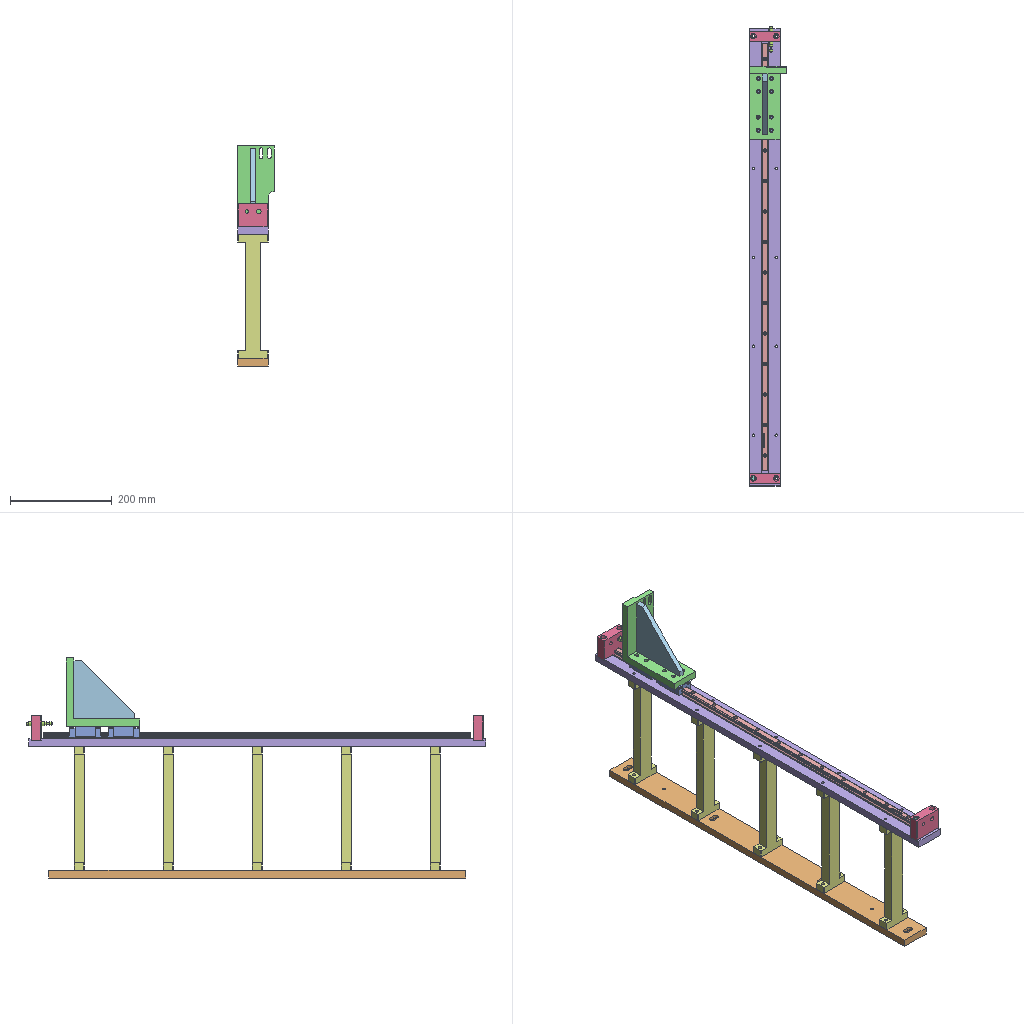Assembly | SolidWorks | 12 different items | 19 placed | box 73 x 905 x 433 mm
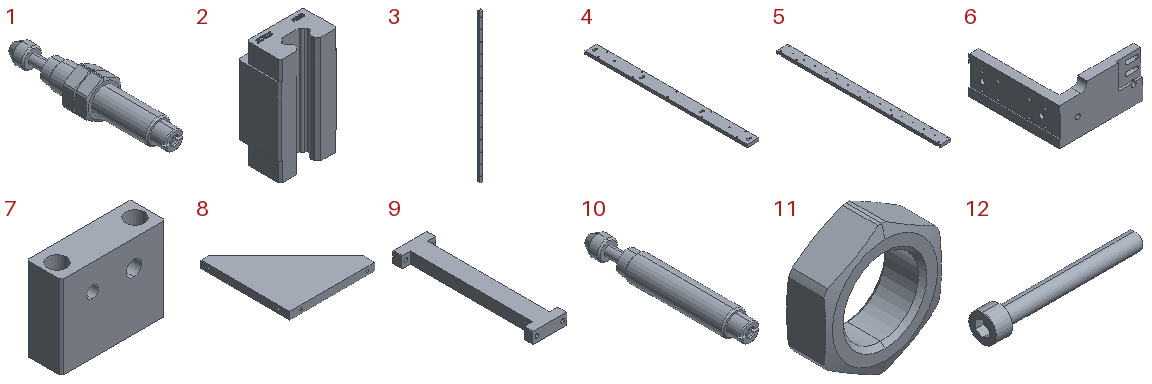Parts list (item | name | quantity | parent item | size | volume | features):
1 | (subassembly) | x1 | - | 11 x 52 x 12.325 mm | 2543 mm3 | -
2 | - | x2 | - | 34 x 23.7 x 61.7 mm | 37046 mm3 | features BaseBody 1
3 | - | x1 | - | 15 x 15 x 840 mm | 154798 mm3 | features Extrusion 1, HoleWzd 1, ICE 1, LPattern 1
4 | - | x1 | - | 60 x 820 x 15 mm | 725646 mm3 | features HoleWzd 3, ICE 2, Extrusion 1, LPattern 1
5 | - | x1 | - | 60 x 900 x 15 mm | 771856 mm3 | features HoleWzd 4, ICE 2, LPattern 2, Extrusion 1
6 | - | x1 | - | 135 x 145 x 72.5 mm | 232445 mm3 | features HoleWzd 4, ICE 4, Fillet 2, ExtruThin 1, Gusset 1
7 | - | x2 | - | 60 x 20 x 48 mm | 51248 mm3 | features HoleWzd 3, Chamfer 1, Extrusion 1
8 | - | x1 | - | 115 x 120 x 10 mm | 82518 mm3 | features HoleWzd 4, ICE 4, Fillet 2, ExtruThin 1, Gusset 1
9 | - | x5 | - | 60 x 244 x 20 mm | 162287 mm3 | features Chamfer 1, Extrusion 1, HoleWzd 1, ICE 1
10 | - | x1 | in 1 | 8 x 52 x 8 mm | 2052 mm3 | features BaseBody 1
11 | - | x2 | in 1 | 11 x 4 x 12.325 mm | 245.478 mm3 | features BaseBody 1
12 | - | x1 | - | 56 x 10 x 10 mm | 1818 mm3 | features BlendCut 1, Cut 1, Fillet 1, LPattern 1, RevCut 1, Revolution 1
Mates (type | each side: item.copy, entity, surface, feature):
Coincident | 5.1 face plane Cut-Extrude3 | 3.1 face plane Boss-Extrude1
Width | 3.1 face plane Boss-Extrude1 | 3.1 face plane Boss-Extrude1 | 5.1 face plane Boss-Extrude1 | 5.1 face plane Boss-Extrude1
DistanceDim | 5.1 face plane Boss-Extrude1 | 3.1 face plane Boss-Extrude1
Coincident | 3.1 face plane Boss-Extrude1 | 2.1 face plane Input1
Width | 2.1 face plane Input1 | 2.1 face plane Input1 | 3.1 face plane Boss-Extrude1 | 3.1 face plane Boss-Extrude1
Coincident | 6.1 face plane Cut-Extrude2 | 2.1 face plane Input1
Width | 6.1 face plane Extrude-Thin1 | 6.1 face plane Extrude-Thin1 | 2.2 face plane Input1 | 2.2 face plane Input1
Concentric | 2.1 face cylinder Input1 | 6.1 face cylinder CBORE for M4 Hex Socket Head Cap Screw1
Coincident | 5.1 face plane Cut-Extrude2 | 7.1 face plane Boss-Extrude1 | 2 times
Coincident | 5.1 face plane Boss-Extrude1 | 7.1 face plane Boss-Extrude1
Coincident | 5.1 face plane Cut-Extrude2 | 7.2 face plane Boss-Extrude1 | 2 times
Coincident | 5.1 face plane Boss-Extrude1 | 7.2 face plane Boss-Extrude1
LimitDistanceDim | 6.1 face plane Extrude-Thin1 | 7.2 face plane Boss-Extrude1
Concentric | 7.1 face cylinder M10x1.0 Tapped Hole1 | 10.1 face cylinder Input1
DistanceDim | 7.1 face plane Boss-Extrude1 | 10.1 face plane Input1
Concentric | 7.2 face cylinder CBORE for M6 Hex Socket Head Cap Screw1 | 12.1 face cylinder Base-Revolve
DistanceDim | 7.2 face plane CBORE for M6 Hex Socket Head Cap Screw1 | 12.1 face plane Base-Revolve
Coincident | 6.1 face plane Extrude-Thin1 | 8.1 face plane Gusset1
Concentric | 6.1 face cylinder CBORE for M4 Hexagon socket head cap screws2 | 8.1 face cylinder M4 Tapped Hole2
Parallel | 6.1 face plane Extrude-Thin1 | 8.1 face plane Gusset1
Coincident | 4.1 face plane Boss-Extrude1 | 9.1 face plane Boss-Extrude1
Coincident | 4.1 face plane Boss-Extrude1 | 9.1 edge
Concentric | 4.1 face cylinder LPattern1 | 9.1 face cylinder M6 Clearance Hole1
Coincident | 5.1 face plane Boss-Extrude1 | 9.1 face plane Boss-Extrude1
Concentric | 5.1 face cylinder LPattern2 | 9.1 face cylinder M6 Clearance Hole1 | 2 times